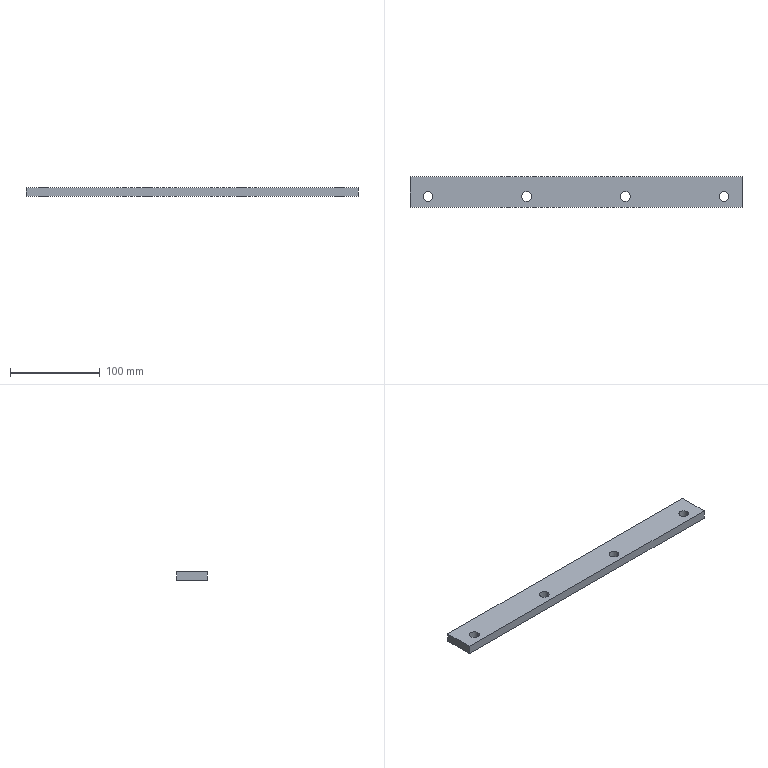Part | SolidWorks | features Extrusion 1 | 1 solid | 14 faces | box 370 x 34 x 10 mm | volume 121999 mm3 | cylinder 8 | plane 6 | commonest cylinder face diameters 11 x8
STEP:
#1=CARTESIAN_POINT('',(-170.5,-5.,10.));
#2=VERTEX_POINT('',#1);
#3=CARTESIAN_POINT('',(-159.5,-5.,10.));
#4=VERTEX_POINT('',#3);
#5=CARTESIAN_POINT('',(-165.,-5.,10.));
#6=DIRECTION('',(0.,0.,1.));
#7=DIRECTION('',(1.,0.,0.));
#8=AXIS2_PLACEMENT_3D('',#5,#6,#7);
#9=CIRCLE('',#8,5.5);
#10=EDGE_CURVE('',#2,#4,#9,.T.);
#11=ORIENTED_EDGE('',*,*,#10,.T.);
#12=CARTESIAN_POINT('',(-159.5,-5.,0.));
#13=VERTEX_POINT('',#12);
#14=CARTESIAN_POINT('',(-159.5,-5.,10.));
#15=DIRECTION('',(0.,0.,-1.));
#16=VECTOR('',#15,1000.);
#17=LINE('',#14,#16);
#18=EDGE_CURVE('',#4,#13,#17,.T.);
#19=ORIENTED_EDGE('',*,*,#18,.T.);
#20=CARTESIAN_POINT('',(-170.5,-5.,0.));
#21=VERTEX_POINT('',#20);
#22=CARTESIAN_POINT('',(-165.,-5.,0.));
#23=DIRECTION('',(0.,0.,1.));
#24=DIRECTION('',(1.,0.,0.));
#25=AXIS2_PLACEMENT_3D('',#22,#23,#24);
#26=CIRCLE('',#25,5.5);
#27=EDGE_CURVE('',#21,#13,#26,.T.);
#28=ORIENTED_EDGE('',*,*,#27,.F.);
#29=CARTESIAN_POINT('',(-170.5,-5.,10.));
#30=DIRECTION('',(0.,0.,-1.));
#31=VECTOR('',#30,1000.);
#32=LINE('',#29,#31);
#33=EDGE_CURVE('',#2,#21,#32,.T.);
#34=ORIENTED_EDGE('',*,*,#33,.F.);
#35=EDGE_LOOP('',(#11,#19,#28,#34));
#36=FACE_OUTER_BOUND('',#35,.T.);
#37=CARTESIAN_POINT('',(-165.,-5.,10.));
#38=DIRECTION('',(0.,0.,-1.));
#39=DIRECTION('',(-1.,0.,0.));
#40=AXIS2_PLACEMENT_3D('',#37,#38,#39);
#41=CYLINDRICAL_SURFACE('',#40,5.5);
#42=ADVANCED_FACE('',(#36),#41,.F.);
#43=CARTESIAN_POINT('',(-60.5,-5.,10.));
#44=VERTEX_POINT('',#43);
#45=CARTESIAN_POINT('',(-49.5,-5.,10.));
#46=VERTEX_POINT('',#45);
#47=CARTESIAN_POINT('',(-55.,-5.,10.));
#48=DIRECTION('',(0.,0.,1.));
#49=DIRECTION('',(1.,0.,0.));
#50=AXIS2_PLACEMENT_3D('',#47,#48,#49);
#51=CIRCLE('',#50,5.5);
#52=EDGE_CURVE('',#44,#46,#51,.T.);
#53=ORIENTED_EDGE('',*,*,#52,.T.);
#54=CARTESIAN_POINT('',(-49.5,-5.,0.));
#55=VERTEX_POINT('',#54);
#56=CARTESIAN_POINT('',(-49.5,-5.,10.));
#57=DIRECTION('',(0.,0.,-1.));
#58=VECTOR('',#57,1000.);
#59=LINE('',#56,#58);
#60=EDGE_CURVE('',#46,#55,#59,.T.);
#61=ORIENTED_EDGE('',*,*,#60,.T.);
#62=CARTESIAN_POINT('',(-60.5,-5.,0.));
#63=VERTEX_POINT('',#62);
#64=CARTESIAN_POINT('',(-55.,-5.,0.));
#65=DIRECTION('',(0.,0.,1.));
#66=DIRECTION('',(1.,0.,0.));
#67=AXIS2_PLACEMENT_3D('',#64,#65,#66);
#68=CIRCLE('',#67,5.5);
#69=EDGE_CURVE('',#63,#55,#68,.T.);
#70=ORIENTED_EDGE('',*,*,#69,.F.);
#71=CARTESIAN_POINT('',(-60.5,-5.,10.));
#72=DIRECTION('',(0.,0.,-1.));
#73=VECTOR('',#72,1000.);
#74=LINE('',#71,#73);
#75=EDGE_CURVE('',#44,#63,#74,.T.);
#76=ORIENTED_EDGE('',*,*,#75,.F.);
#77=EDGE_LOOP('',(#53,#61,#70,#76));
#78=FACE_OUTER_BOUND('',#77,.T.);
#79=CARTESIAN_POINT('',(-55.,-5.,10.));
#80=DIRECTION('',(0.,0.,-1.));
#81=DIRECTION('',(-1.,0.,0.));
#82=AXIS2_PLACEMENT_3D('',#79,#80,#81);
#83=CYLINDRICAL_SURFACE('',#82,5.5);
#84=ADVANCED_FACE('',(#78),#83,.F.);
#85=CARTESIAN_POINT('',(49.5,-5.,10.));
#86=VERTEX_POINT('',#85);
#87=CARTESIAN_POINT('',(60.5,-5.,10.));
#88=VERTEX_POINT('',#87);
#89=CARTESIAN_POINT('',(55.,-5.,10.));
#90=DIRECTION('',(0.,0.,1.));
#91=DIRECTION('',(1.,0.,0.));
#92=AXIS2_PLACEMENT_3D('',#89,#90,#91);
#93=CIRCLE('',#92,5.5);
#94=EDGE_CURVE('',#86,#88,#93,.T.);
#95=ORIENTED_EDGE('',*,*,#94,.T.);
#96=CARTESIAN_POINT('',(60.5,-5.,0.));
#97=VERTEX_POINT('',#96);
#98=CARTESIAN_POINT('',(60.5,-5.,10.));
#99=DIRECTION('',(0.,0.,-1.));
#100=VECTOR('',#99,1000.);
#101=LINE('',#98,#100);
#102=EDGE_CURVE('',#88,#97,#101,.T.);
#103=ORIENTED_EDGE('',*,*,#102,.T.);
#104=CARTESIAN_POINT('',(49.5,-5.,0.));
#105=VERTEX_POINT('',#104);
#106=CARTESIAN_POINT('',(55.,-5.,0.));
#107=DIRECTION('',(0.,0.,1.));
#108=DIRECTION('',(1.,0.,0.));
#109=AXIS2_PLACEMENT_3D('',#106,#107,#108);
#110=CIRCLE('',#109,5.5);
#111=EDGE_CURVE('',#105,#97,#110,.T.);
#112=ORIENTED_EDGE('',*,*,#111,.F.);
#113=CARTESIAN_POINT('',(49.5,-5.,10.));
#114=DIRECTION('',(0.,0.,-1.));
#115=VECTOR('',#114,1000.);
#116=LINE('',#113,#115);
#117=EDGE_CURVE('',#86,#105,#116,.T.);
#118=ORIENTED_EDGE('',*,*,#117,.F.);
#119=EDGE_LOOP('',(#95,#103,#112,#118));
#120=FACE_OUTER_BOUND('',#119,.T.);
#121=CARTESIAN_POINT('',(55.,-5.,10.));
#122=DIRECTION('',(0.,0.,-1.));
#123=DIRECTION('',(-1.,0.,0.));
#124=AXIS2_PLACEMENT_3D('',#121,#122,#123);
#125=CYLINDRICAL_SURFACE('',#124,5.5);
#126=ADVANCED_FACE('',(#120),#125,.F.);
#127=CARTESIAN_POINT('',(159.5,-5.,10.));
#128=VERTEX_POINT('',#127);
#129=CARTESIAN_POINT('',(170.5,-5.,10.));
#130=VERTEX_POINT('',#129);
#131=CARTESIAN_POINT('',(165.,-5.,10.));
#132=DIRECTION('',(0.,0.,1.));
#133=DIRECTION('',(1.,0.,0.));
#134=AXIS2_PLACEMENT_3D('',#131,#132,#133);
#135=CIRCLE('',#134,5.5);
#136=EDGE_CURVE('',#128,#130,#135,.T.);
#137=ORIENTED_EDGE('',*,*,#136,.T.);
#138=CARTESIAN_POINT('',(170.5,-5.,0.));
#139=VERTEX_POINT('',#138);
#140=CARTESIAN_POINT('',(170.5,-5.,10.));
#141=DIRECTION('',(0.,0.,-1.));
#142=VECTOR('',#141,1000.);
#143=LINE('',#140,#142);
#144=EDGE_CURVE('',#130,#139,#143,.T.);
#145=ORIENTED_EDGE('',*,*,#144,.T.);
#146=CARTESIAN_POINT('',(159.5,-5.,0.));
#147=VERTEX_POINT('',#146);
#148=CARTESIAN_POINT('',(165.,-5.,0.));
#149=DIRECTION('',(0.,0.,1.));
#150=DIRECTION('',(1.,0.,0.));
#151=AXIS2_PLACEMENT_3D('',#148,#149,#150);
#152=CIRCLE('',#151,5.5);
#153=EDGE_CURVE('',#147,#139,#152,.T.);
#154=ORIENTED_EDGE('',*,*,#153,.F.);
#155=CARTESIAN_POINT('',(159.5,-5.,10.));
#156=DIRECTION('',(0.,0.,-1.));
#157=VECTOR('',#156,1000.);
#158=LINE('',#155,#157);
#159=EDGE_CURVE('',#128,#147,#158,.T.);
#160=ORIENTED_EDGE('',*,*,#159,.F.);
#161=EDGE_LOOP('',(#137,#145,#154,#160));
#162=FACE_OUTER_BOUND('',#161,.T.);
#163=CARTESIAN_POINT('',(165.,-5.,10.));
#164=DIRECTION('',(0.,0.,-1.));
#165=DIRECTION('',(-1.,0.,0.));
#166=AXIS2_PLACEMENT_3D('',#163,#164,#165);
#167=CYLINDRICAL_SURFACE('',#166,5.5);
#168=ADVANCED_FACE('',(#162),#167,.F.);
#169=CARTESIAN_POINT('',(185.,-17.,10.));
#170=VERTEX_POINT('',#169);
#171=CARTESIAN_POINT('',(185.,17.,10.));
#172=VERTEX_POINT('',#171);
#173=CARTESIAN_POINT('',(185.,-17.,10.));
#174=DIRECTION('',(0.,1.,0.));
#175=VECTOR('',#174,1000.);
#176=LINE('',#173,#175);
#177=EDGE_CURVE('',#170,#172,#176,.T.);
#178=ORIENTED_EDGE('',*,*,#177,.T.);
#179=CARTESIAN_POINT('',(-185.,17.,10.));
#180=VERTEX_POINT('',#179);
#181=CARTESIAN_POINT('',(-185.,17.,10.));
#182=DIRECTION('',(-1.,0.,0.));
#183=VECTOR('',#182,1000.);
#184=LINE('',#181,#183);
#185=EDGE_CURVE('',#172,#180,#184,.T.);
#186=ORIENTED_EDGE('',*,*,#185,.T.);
#187=CARTESIAN_POINT('',(-185.,-17.,10.));
#188=VERTEX_POINT('',#187);
#189=CARTESIAN_POINT('',(-185.,-17.,10.));
#190=DIRECTION('',(0.,-1.,0.));
#191=VECTOR('',#190,1000.);
#192=LINE('',#189,#191);
#193=EDGE_CURVE('',#180,#188,#192,.T.);
#194=ORIENTED_EDGE('',*,*,#193,.T.);
#195=CARTESIAN_POINT('',(-185.,-17.,10.));
#196=DIRECTION('',(1.,0.,0.));
#197=VECTOR('',#196,1000.);
#198=LINE('',#195,#197);
#199=EDGE_CURVE('',#188,#170,#198,.T.);
#200=ORIENTED_EDGE('',*,*,#199,.T.);
#201=EDGE_LOOP('',(#178,#186,#194,#200));
#202=FACE_OUTER_BOUND('',#201,.T.);
#203=ORIENTED_EDGE('',*,*,#136,.F.);
#204=CARTESIAN_POINT('',(165.,-5.,10.));
#205=DIRECTION('',(0.,0.,1.));
#206=DIRECTION('',(1.,0.,0.));
#207=AXIS2_PLACEMENT_3D('',#204,#205,#206);
#208=CIRCLE('',#207,5.5);
#209=EDGE_CURVE('',#130,#128,#208,.T.);
#210=ORIENTED_EDGE('',*,*,#209,.F.);
#211=EDGE_LOOP('',(#203,#210));
#212=FACE_BOUND('',#211,.T.);
#213=ORIENTED_EDGE('',*,*,#94,.F.);
#214=CARTESIAN_POINT('',(55.,-5.,10.));
#215=DIRECTION('',(0.,0.,1.));
#216=DIRECTION('',(1.,0.,0.));
#217=AXIS2_PLACEMENT_3D('',#214,#215,#216);
#218=CIRCLE('',#217,5.5);
#219=EDGE_CURVE('',#88,#86,#218,.T.);
#220=ORIENTED_EDGE('',*,*,#219,.F.);
#221=EDGE_LOOP('',(#213,#220));
#222=FACE_BOUND('',#221,.T.);
#223=ORIENTED_EDGE('',*,*,#52,.F.);
#224=CARTESIAN_POINT('',(-55.,-5.,10.));
#225=DIRECTION('',(0.,0.,1.));
#226=DIRECTION('',(1.,0.,0.));
#227=AXIS2_PLACEMENT_3D('',#224,#225,#226);
#228=CIRCLE('',#227,5.5);
#229=EDGE_CURVE('',#46,#44,#228,.T.);
#230=ORIENTED_EDGE('',*,*,#229,.F.);
#231=EDGE_LOOP('',(#223,#230));
#232=FACE_BOUND('',#231,.T.);
#233=ORIENTED_EDGE('',*,*,#10,.F.);
#234=CARTESIAN_POINT('',(-165.,-5.,10.));
#235=DIRECTION('',(0.,0.,1.));
#236=DIRECTION('',(1.,0.,0.));
#237=AXIS2_PLACEMENT_3D('',#234,#235,#236);
#238=CIRCLE('',#237,5.5);
#239=EDGE_CURVE('',#4,#2,#238,.T.);
#240=ORIENTED_EDGE('',*,*,#239,.F.);
#241=EDGE_LOOP('',(#233,#240));
#242=FACE_BOUND('',#241,.T.);
#243=CARTESIAN_POINT('',(0.,0.,10.));
#244=DIRECTION('',(0.,0.,-1.));
#245=DIRECTION('',(-1.,0.,0.));
#246=AXIS2_PLACEMENT_3D('',#243,#244,#245);
#247=PLANE('',#246);
#248=ADVANCED_FACE('',(#202,#212,#222,#232,#242),#247,.F.);
#249=ORIENTED_EDGE('',*,*,#69,.T.);
#250=CARTESIAN_POINT('',(-55.,-5.,0.));
#251=DIRECTION('',(0.,0.,1.));
#252=DIRECTION('',(1.,0.,0.));
#253=AXIS2_PLACEMENT_3D('',#250,#251,#252);
#254=CIRCLE('',#253,5.5);
#255=EDGE_CURVE('',#55,#63,#254,.T.);
#256=ORIENTED_EDGE('',*,*,#255,.T.);
#257=EDGE_LOOP('',(#249,#256));
#258=FACE_BOUND('',#257,.T.);
#259=ORIENTED_EDGE('',*,*,#153,.T.);
#260=CARTESIAN_POINT('',(165.,-5.,0.));
#261=DIRECTION('',(0.,0.,1.));
#262=DIRECTION('',(1.,0.,0.));
#263=AXIS2_PLACEMENT_3D('',#260,#261,#262);
#264=CIRCLE('',#263,5.5);
#265=EDGE_CURVE('',#139,#147,#264,.T.);
#266=ORIENTED_EDGE('',*,*,#265,.T.);
#267=EDGE_LOOP('',(#259,#266));
#268=FACE_BOUND('',#267,.T.);
#269=CARTESIAN_POINT('',(185.,-17.,0.));
#270=VERTEX_POINT('',#269);
#271=CARTESIAN_POINT('',(185.,17.,0.));
#272=VERTEX_POINT('',#271);
#273=CARTESIAN_POINT('',(185.,-17.,0.));
#274=DIRECTION('',(0.,1.,0.));
#275=VECTOR('',#274,1000.);
#276=LINE('',#273,#275);
#277=EDGE_CURVE('',#270,#272,#276,.T.);
#278=ORIENTED_EDGE('',*,*,#277,.F.);
#279=CARTESIAN_POINT('',(-185.,-17.,0.));
#280=VERTEX_POINT('',#279);
#281=CARTESIAN_POINT('',(-185.,-17.,0.));
#282=DIRECTION('',(1.,0.,0.));
#283=VECTOR('',#282,1000.);
#284=LINE('',#281,#283);
#285=EDGE_CURVE('',#280,#270,#284,.T.);
#286=ORIENTED_EDGE('',*,*,#285,.F.);
#287=CARTESIAN_POINT('',(-185.,17.,0.));
#288=VERTEX_POINT('',#287);
#289=CARTESIAN_POINT('',(-185.,-17.,0.));
#290=DIRECTION('',(0.,-1.,0.));
#291=VECTOR('',#290,1000.);
#292=LINE('',#289,#291);
#293=EDGE_CURVE('',#288,#280,#292,.T.);
#294=ORIENTED_EDGE('',*,*,#293,.F.);
#295=CARTESIAN_POINT('',(-185.,17.,0.));
#296=DIRECTION('',(-1.,0.,0.));
#297=VECTOR('',#296,1000.);
#298=LINE('',#295,#297);
#299=EDGE_CURVE('',#272,#288,#298,.T.);
#300=ORIENTED_EDGE('',*,*,#299,.F.);
#301=EDGE_LOOP('',(#278,#286,#294,#300));
#302=FACE_OUTER_BOUND('',#301,.T.);
#303=ORIENTED_EDGE('',*,*,#111,.T.);
#304=CARTESIAN_POINT('',(55.,-5.,0.));
#305=DIRECTION('',(0.,0.,1.));
#306=DIRECTION('',(1.,0.,0.));
#307=AXIS2_PLACEMENT_3D('',#304,#305,#306);
#308=CIRCLE('',#307,5.5);
#309=EDGE_CURVE('',#97,#105,#308,.T.);
#310=ORIENTED_EDGE('',*,*,#309,.T.);
#311=EDGE_LOOP('',(#303,#310));
#312=FACE_BOUND('',#311,.T.);
#313=ORIENTED_EDGE('',*,*,#27,.T.);
#314=CARTESIAN_POINT('',(-165.,-5.,0.));
#315=DIRECTION('',(0.,0.,1.));
#316=DIRECTION('',(1.,0.,0.));
#317=AXIS2_PLACEMENT_3D('',#314,#315,#316);
#318=CIRCLE('',#317,5.5);
#319=EDGE_CURVE('',#13,#21,#318,.T.);
#320=ORIENTED_EDGE('',*,*,#319,.T.);
#321=EDGE_LOOP('',(#313,#320));
#322=FACE_BOUND('',#321,.T.);
#323=CARTESIAN_POINT('',(0.,0.,0.));
#324=DIRECTION('',(0.,0.,-1.));
#325=DIRECTION('',(-1.,0.,0.));
#326=AXIS2_PLACEMENT_3D('',#323,#324,#325);
#327=PLANE('',#326);
#328=ADVANCED_FACE('',(#258,#268,#302,#312,#322),#327,.T.);
#329=ORIENTED_EDGE('',*,*,#277,.T.);
#330=CARTESIAN_POINT('',(185.,17.,10.));
#331=DIRECTION('',(0.,0.,-1.));
#332=VECTOR('',#331,1000.);
#333=LINE('',#330,#332);
#334=EDGE_CURVE('',#172,#272,#333,.T.);
#335=ORIENTED_EDGE('',*,*,#334,.F.);
#336=ORIENTED_EDGE('',*,*,#177,.F.);
#337=CARTESIAN_POINT('',(185.,-17.,10.));
#338=DIRECTION('',(0.,0.,-1.));
#339=VECTOR('',#338,1000.);
#340=LINE('',#337,#339);
#341=EDGE_CURVE('',#170,#270,#340,.T.);
#342=ORIENTED_EDGE('',*,*,#341,.T.);
#343=EDGE_LOOP('',(#329,#335,#336,#342));
#344=FACE_OUTER_BOUND('',#343,.T.);
#345=CARTESIAN_POINT('',(185.,-17.,10.));
#346=DIRECTION('',(-1.,0.,0.));
#347=DIRECTION('',(0.,0.,1.));
#348=AXIS2_PLACEMENT_3D('',#345,#346,#347);
#349=PLANE('',#348);
#350=ADVANCED_FACE('',(#344),#349,.F.);
#351=ORIENTED_EDGE('',*,*,#299,.T.);
#352=CARTESIAN_POINT('',(-185.,17.,10.));
#353=DIRECTION('',(0.,0.,-1.));
#354=VECTOR('',#353,1000.);
#355=LINE('',#352,#354);
#356=EDGE_CURVE('',#180,#288,#355,.T.);
#357=ORIENTED_EDGE('',*,*,#356,.F.);
#358=ORIENTED_EDGE('',*,*,#185,.F.);
#359=ORIENTED_EDGE('',*,*,#334,.T.);
#360=EDGE_LOOP('',(#351,#357,#358,#359));
#361=FACE_OUTER_BOUND('',#360,.T.);
#362=CARTESIAN_POINT('',(-185.,17.,10.));
#363=DIRECTION('',(0.,-1.,0.));
#364=DIRECTION('',(0.,0.,-1.));
#365=AXIS2_PLACEMENT_3D('',#362,#363,#364);
#366=PLANE('',#365);
#367=ADVANCED_FACE('',(#361),#366,.F.);
#368=ORIENTED_EDGE('',*,*,#293,.T.);
#369=CARTESIAN_POINT('',(-185.,-17.,10.));
#370=DIRECTION('',(0.,0.,-1.));
#371=VECTOR('',#370,1000.);
#372=LINE('',#369,#371);
#373=EDGE_CURVE('',#188,#280,#372,.T.);
#374=ORIENTED_EDGE('',*,*,#373,.F.);
#375=ORIENTED_EDGE('',*,*,#193,.F.);
#376=ORIENTED_EDGE('',*,*,#356,.T.);
#377=EDGE_LOOP('',(#368,#374,#375,#376));
#378=FACE_OUTER_BOUND('',#377,.T.);
#379=CARTESIAN_POINT('',(-185.,-17.,10.));
#380=DIRECTION('',(1.,0.,0.));
#381=DIRECTION('',(0.,0.,-1.));
#382=AXIS2_PLACEMENT_3D('',#379,#380,#381);
#383=PLANE('',#382);
#384=ADVANCED_FACE('',(#378),#383,.F.);
#385=ORIENTED_EDGE('',*,*,#285,.T.);
#386=ORIENTED_EDGE('',*,*,#341,.F.);
#387=ORIENTED_EDGE('',*,*,#199,.F.);
#388=ORIENTED_EDGE('',*,*,#373,.T.);
#389=EDGE_LOOP('',(#385,#386,#387,#388));
#390=FACE_OUTER_BOUND('',#389,.T.);
#391=CARTESIAN_POINT('',(-185.,-17.,10.));
#392=DIRECTION('',(0.,1.,0.));
#393=DIRECTION('',(0.,0.,1.));
#394=AXIS2_PLACEMENT_3D('',#391,#392,#393);
#395=PLANE('',#394);
#396=ADVANCED_FACE('',(#390),#395,.F.);
#397=ORIENTED_EDGE('',*,*,#144,.F.);
#398=ORIENTED_EDGE('',*,*,#209,.T.);
#399=ORIENTED_EDGE('',*,*,#159,.T.);
#400=ORIENTED_EDGE('',*,*,#265,.F.);
#401=EDGE_LOOP('',(#397,#398,#399,#400));
#402=FACE_OUTER_BOUND('',#401,.T.);
#403=CARTESIAN_POINT('',(165.,-5.,10.));
#404=DIRECTION('',(0.,0.,-1.));
#405=DIRECTION('',(-1.,0.,0.));
#406=AXIS2_PLACEMENT_3D('',#403,#404,#405);
#407=CYLINDRICAL_SURFACE('',#406,5.5);
#408=ADVANCED_FACE('',(#402),#407,.F.);
#409=ORIENTED_EDGE('',*,*,#102,.F.);
#410=ORIENTED_EDGE('',*,*,#219,.T.);
#411=ORIENTED_EDGE('',*,*,#117,.T.);
#412=ORIENTED_EDGE('',*,*,#309,.F.);
#413=EDGE_LOOP('',(#409,#410,#411,#412));
#414=FACE_OUTER_BOUND('',#413,.T.);
#415=CARTESIAN_POINT('',(55.,-5.,10.));
#416=DIRECTION('',(0.,0.,-1.));
#417=DIRECTION('',(-1.,0.,0.));
#418=AXIS2_PLACEMENT_3D('',#415,#416,#417);
#419=CYLINDRICAL_SURFACE('',#418,5.5);
#420=ADVANCED_FACE('',(#414),#419,.F.);
#421=ORIENTED_EDGE('',*,*,#60,.F.);
#422=ORIENTED_EDGE('',*,*,#229,.T.);
#423=ORIENTED_EDGE('',*,*,#75,.T.);
#424=ORIENTED_EDGE('',*,*,#255,.F.);
#425=EDGE_LOOP('',(#421,#422,#423,#424));
#426=FACE_OUTER_BOUND('',#425,.T.);
#427=CARTESIAN_POINT('',(-55.,-5.,10.));
#428=DIRECTION('',(0.,0.,-1.));
#429=DIRECTION('',(-1.,0.,0.));
#430=AXIS2_PLACEMENT_3D('',#427,#428,#429);
#431=CYLINDRICAL_SURFACE('',#430,5.5);
#432=ADVANCED_FACE('',(#426),#431,.F.);
#433=ORIENTED_EDGE('',*,*,#18,.F.);
#434=ORIENTED_EDGE('',*,*,#239,.T.);
#435=ORIENTED_EDGE('',*,*,#33,.T.);
#436=ORIENTED_EDGE('',*,*,#319,.F.);
#437=EDGE_LOOP('',(#433,#434,#435,#436));
#438=FACE_OUTER_BOUND('',#437,.T.);
#439=CARTESIAN_POINT('',(-165.,-5.,10.));
#440=DIRECTION('',(0.,0.,-1.));
#441=DIRECTION('',(-1.,0.,0.));
#442=AXIS2_PLACEMENT_3D('',#439,#440,#441);
#443=CYLINDRICAL_SURFACE('',#442,5.5);
#444=ADVANCED_FACE('',(#438),#443,.F.);
#445=CLOSED_SHELL('',(#42,#84,#126,#168,#248,#328,#350,#367,#384,#396,#408,#420,#432,#444));
#446=MANIFOLD_SOLID_BREP('',#445);
#447=CARTESIAN_POINT('',(0.,0.,0.));
#448=DIRECTION('',(0.,0.,1.));
#449=DIRECTION('',(1.,0.,0.));
#450=AXIS2_PLACEMENT_3D('',#447,#448,#449);
#451=(LENGTH_UNIT()NAMED_UNIT(*)SI_UNIT(.MILLI.,.METRE.));
#452=UNCERTAINTY_MEASURE_WITH_UNIT(LENGTH_MEASURE(0.00001),#451,'','');
#453=(NAMED_UNIT(*)PLANE_ANGLE_UNIT()SI_UNIT($,.RADIAN.));
#454=(NAMED_UNIT(*)SI_UNIT($,.STERADIAN.)SOLID_ANGLE_UNIT());
#455=(GEOMETRIC_REPRESENTATION_CONTEXT(3)GLOBAL_UNCERTAINTY_ASSIGNED_CONTEXT((#452))GLOBAL_UNIT_ASSIGNED_CONTEXT((#451,#453,#454))REPRESENTATION_CONTEXT('',''));
#456=ADVANCED_BREP_SHAPE_REPRESENTATION('',(#446,#450),#455);